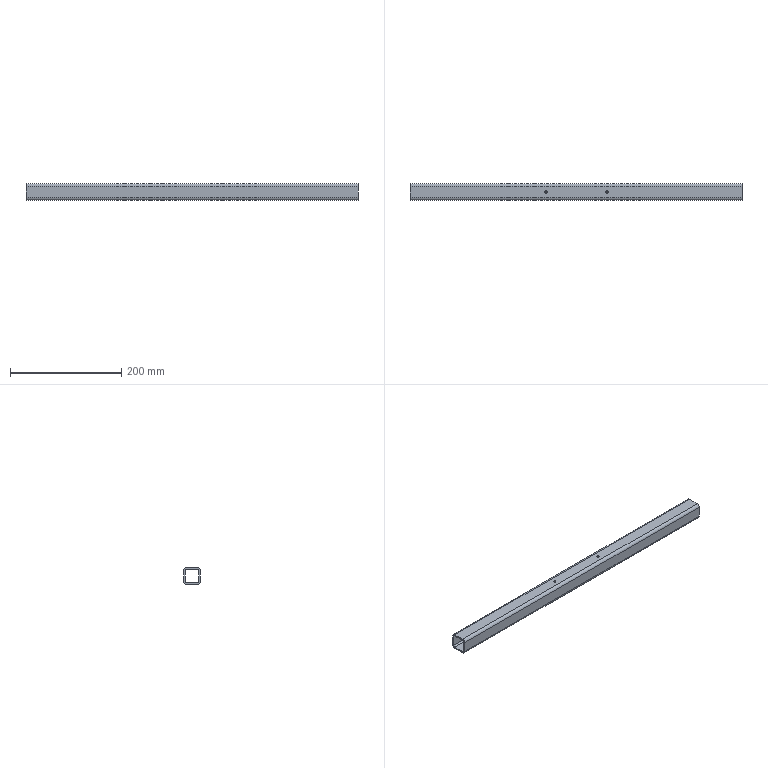Part | SolidWorks | features 3DProfileFeature 1, HoleWzd 1, WeldMemberFeat 1, WeldmentFeature 1 | 1 solid | 26 faces | box 598 x 30 x 30 mm | volume 159852 mm3 | cylinder 16 | plane 10 | commonest cylinder face diameters 4.2 x8 5.2 x4 10.4 x4
STEP:
#1=CARTESIAN_POINT('',(357.1,0.,12.4));
#2=VERTEX_POINT('',#1);
#3=CARTESIAN_POINT('',(352.9,0.,12.4));
#4=VERTEX_POINT('',#3);
#5=CARTESIAN_POINT('',(355.,0.,12.4));
#6=DIRECTION('',(0.,0.,-1.));
#7=DIRECTION('',(-1.,0.,0.));
#8=AXIS2_PLACEMENT_3D('',#5,#6,#7);
#9=CIRCLE('',#8,2.1);
#10=EDGE_CURVE('',#2,#4,#9,.T.);
#11=ORIENTED_EDGE('',*,*,#10,.T.);
#12=CARTESIAN_POINT('',(352.9,0.,15.));
#13=VERTEX_POINT('',#12);
#14=CARTESIAN_POINT('',(352.9,0.,15.));
#15=DIRECTION('',(0.,0.,1.));
#16=VECTOR('',#15,1000.);
#17=LINE('',#14,#16);
#18=EDGE_CURVE('',#4,#13,#17,.T.);
#19=ORIENTED_EDGE('',*,*,#18,.T.);
#20=CARTESIAN_POINT('',(357.1,0.,15.));
#21=VERTEX_POINT('',#20);
#22=CARTESIAN_POINT('',(355.,0.,15.));
#23=DIRECTION('',(0.,0.,1.));
#24=DIRECTION('',(1.,0.,0.));
#25=AXIS2_PLACEMENT_3D('',#22,#23,#24);
#26=CIRCLE('',#25,2.1);
#27=EDGE_CURVE('',#13,#21,#26,.T.);
#28=ORIENTED_EDGE('',*,*,#27,.T.);
#29=CARTESIAN_POINT('',(357.1,0.,15.));
#30=DIRECTION('',(0.,0.,1.));
#31=VECTOR('',#30,1000.);
#32=LINE('',#29,#31);
#33=EDGE_CURVE('',#2,#21,#32,.T.);
#34=ORIENTED_EDGE('',*,*,#33,.F.);
#35=EDGE_LOOP('',(#11,#19,#28,#34));
#36=FACE_OUTER_BOUND('',#35,.T.);
#37=CARTESIAN_POINT('',(355.,0.,15.));
#38=DIRECTION('',(0.,0.,1.));
#39=DIRECTION('',(1.,0.,0.));
#40=AXIS2_PLACEMENT_3D('',#37,#38,#39);
#41=CYLINDRICAL_SURFACE('',#40,2.1);
#42=ADVANCED_FACE('',(#36),#41,.F.);
#43=CARTESIAN_POINT('',(352.9,0.,-15.));
#44=VERTEX_POINT('',#43);
#45=CARTESIAN_POINT('',(357.1,0.,-15.));
#46=VERTEX_POINT('',#45);
#47=CARTESIAN_POINT('',(355.,0.,-15.));
#48=DIRECTION('',(0.,0.,1.));
#49=DIRECTION('',(1.,0.,0.));
#50=AXIS2_PLACEMENT_3D('',#47,#48,#49);
#51=CIRCLE('',#50,2.1);
#52=EDGE_CURVE('',#44,#46,#51,.T.);
#53=ORIENTED_EDGE('',*,*,#52,.F.);
#54=CARTESIAN_POINT('',(352.9,0.,-12.4));
#55=VERTEX_POINT('',#54);
#56=CARTESIAN_POINT('',(352.9,0.,15.));
#57=DIRECTION('',(0.,0.,1.));
#58=VECTOR('',#57,1000.);
#59=LINE('',#56,#58);
#60=EDGE_CURVE('',#44,#55,#59,.T.);
#61=ORIENTED_EDGE('',*,*,#60,.T.);
#62=CARTESIAN_POINT('',(357.1,0.,-12.4));
#63=VERTEX_POINT('',#62);
#64=CARTESIAN_POINT('',(355.,0.,-12.4));
#65=DIRECTION('',(0.,0.,1.));
#66=DIRECTION('',(1.,0.,0.));
#67=AXIS2_PLACEMENT_3D('',#64,#65,#66);
#68=CIRCLE('',#67,2.1);
#69=EDGE_CURVE('',#55,#63,#68,.T.);
#70=ORIENTED_EDGE('',*,*,#69,.T.);
#71=CARTESIAN_POINT('',(357.1,0.,15.));
#72=DIRECTION('',(0.,0.,1.));
#73=VECTOR('',#72,1000.);
#74=LINE('',#71,#73);
#75=EDGE_CURVE('',#46,#63,#74,.T.);
#76=ORIENTED_EDGE('',*,*,#75,.F.);
#77=EDGE_LOOP('',(#53,#61,#70,#76));
#78=FACE_OUTER_BOUND('',#77,.T.);
#79=CARTESIAN_POINT('',(355.,0.,15.));
#80=DIRECTION('',(0.,0.,1.));
#81=DIRECTION('',(1.,0.,0.));
#82=AXIS2_PLACEMENT_3D('',#79,#80,#81);
#83=CYLINDRICAL_SURFACE('',#82,2.1);
#84=ADVANCED_FACE('',(#78),#83,.F.);
#85=CARTESIAN_POINT('',(247.1,0.,12.4));
#86=VERTEX_POINT('',#85);
#87=CARTESIAN_POINT('',(242.9,0.,12.4));
#88=VERTEX_POINT('',#87);
#89=CARTESIAN_POINT('',(245.,0.,12.4));
#90=DIRECTION('',(0.,0.,-1.));
#91=DIRECTION('',(-1.,0.,0.));
#92=AXIS2_PLACEMENT_3D('',#89,#90,#91);
#93=CIRCLE('',#92,2.1);
#94=EDGE_CURVE('',#86,#88,#93,.T.);
#95=ORIENTED_EDGE('',*,*,#94,.T.);
#96=CARTESIAN_POINT('',(242.9,0.,15.));
#97=VERTEX_POINT('',#96);
#98=CARTESIAN_POINT('',(242.9,0.,15.));
#99=DIRECTION('',(0.,0.,1.));
#100=VECTOR('',#99,1000.);
#101=LINE('',#98,#100);
#102=EDGE_CURVE('',#88,#97,#101,.T.);
#103=ORIENTED_EDGE('',*,*,#102,.T.);
#104=CARTESIAN_POINT('',(247.1,0.,15.));
#105=VERTEX_POINT('',#104);
#106=CARTESIAN_POINT('',(245.,0.,15.));
#107=DIRECTION('',(0.,0.,1.));
#108=DIRECTION('',(1.,0.,0.));
#109=AXIS2_PLACEMENT_3D('',#106,#107,#108);
#110=CIRCLE('',#109,2.1);
#111=EDGE_CURVE('',#97,#105,#110,.T.);
#112=ORIENTED_EDGE('',*,*,#111,.T.);
#113=CARTESIAN_POINT('',(247.1,0.,15.));
#114=DIRECTION('',(0.,0.,1.));
#115=VECTOR('',#114,1000.);
#116=LINE('',#113,#115);
#117=EDGE_CURVE('',#86,#105,#116,.T.);
#118=ORIENTED_EDGE('',*,*,#117,.F.);
#119=EDGE_LOOP('',(#95,#103,#112,#118));
#120=FACE_OUTER_BOUND('',#119,.T.);
#121=CARTESIAN_POINT('',(245.,0.,15.));
#122=DIRECTION('',(0.,0.,1.));
#123=DIRECTION('',(1.,0.,0.));
#124=AXIS2_PLACEMENT_3D('',#121,#122,#123);
#125=CYLINDRICAL_SURFACE('',#124,2.1);
#126=ADVANCED_FACE('',(#120),#125,.F.);
#127=CARTESIAN_POINT('',(242.9,0.,-15.));
#128=VERTEX_POINT('',#127);
#129=CARTESIAN_POINT('',(247.1,0.,-15.));
#130=VERTEX_POINT('',#129);
#131=CARTESIAN_POINT('',(245.,0.,-15.));
#132=DIRECTION('',(0.,0.,1.));
#133=DIRECTION('',(1.,0.,0.));
#134=AXIS2_PLACEMENT_3D('',#131,#132,#133);
#135=CIRCLE('',#134,2.1);
#136=EDGE_CURVE('',#128,#130,#135,.T.);
#137=ORIENTED_EDGE('',*,*,#136,.F.);
#138=CARTESIAN_POINT('',(242.9,0.,-12.4));
#139=VERTEX_POINT('',#138);
#140=CARTESIAN_POINT('',(242.9,0.,15.));
#141=DIRECTION('',(0.,0.,1.));
#142=VECTOR('',#141,1000.);
#143=LINE('',#140,#142);
#144=EDGE_CURVE('',#128,#139,#143,.T.);
#145=ORIENTED_EDGE('',*,*,#144,.T.);
#146=CARTESIAN_POINT('',(247.1,0.,-12.4));
#147=VERTEX_POINT('',#146);
#148=CARTESIAN_POINT('',(245.,0.,-12.4));
#149=DIRECTION('',(0.,0.,1.));
#150=DIRECTION('',(1.,0.,0.));
#151=AXIS2_PLACEMENT_3D('',#148,#149,#150);
#152=CIRCLE('',#151,2.1);
#153=EDGE_CURVE('',#139,#147,#152,.T.);
#154=ORIENTED_EDGE('',*,*,#153,.T.);
#155=CARTESIAN_POINT('',(247.1,0.,15.));
#156=DIRECTION('',(0.,0.,1.));
#157=VECTOR('',#156,1000.);
#158=LINE('',#155,#157);
#159=EDGE_CURVE('',#130,#147,#158,.T.);
#160=ORIENTED_EDGE('',*,*,#159,.F.);
#161=EDGE_LOOP('',(#137,#145,#154,#160));
#162=FACE_OUTER_BOUND('',#161,.T.);
#163=CARTESIAN_POINT('',(245.,0.,15.));
#164=DIRECTION('',(0.,0.,1.));
#165=DIRECTION('',(1.,0.,0.));
#166=AXIS2_PLACEMENT_3D('',#163,#164,#165);
#167=CYLINDRICAL_SURFACE('',#166,2.1);
#168=ADVANCED_FACE('',(#162),#167,.F.);
#169=CARTESIAN_POINT('',(0.,9.8,-15.));
#170=VERTEX_POINT('',#169);
#171=CARTESIAN_POINT('',(0.,15.,-9.8));
#172=VERTEX_POINT('',#171);
#173=CARTESIAN_POINT('',(0.,9.8,-9.8));
#174=DIRECTION('',(1.,0.,0.));
#175=DIRECTION('',(0.,0.,-1.));
#176=AXIS2_PLACEMENT_3D('',#173,#174,#175);
#177=CIRCLE('',#176,5.2);
#178=EDGE_CURVE('',#170,#172,#177,.T.);
#179=ORIENTED_EDGE('',*,*,#178,.T.);
#180=CARTESIAN_POINT('',(598.,15.,-9.8));
#181=VERTEX_POINT('',#180);
#182=CARTESIAN_POINT('',(598.,15.,-9.8));
#183=DIRECTION('',(-1.,0.,0.));
#184=VECTOR('',#183,1000.);
#185=LINE('',#182,#184);
#186=EDGE_CURVE('',#181,#172,#185,.T.);
#187=ORIENTED_EDGE('',*,*,#186,.F.);
#188=CARTESIAN_POINT('',(598.,9.8,-15.));
#189=VERTEX_POINT('',#188);
#190=CARTESIAN_POINT('',(598.,9.8,-9.8));
#191=DIRECTION('',(1.,0.,0.));
#192=DIRECTION('',(0.,0.,-1.));
#193=AXIS2_PLACEMENT_3D('',#190,#191,#192);
#194=CIRCLE('',#193,5.2);
#195=EDGE_CURVE('',#189,#181,#194,.T.);
#196=ORIENTED_EDGE('',*,*,#195,.F.);
#197=CARTESIAN_POINT('',(598.,9.8,-15.));
#198=DIRECTION('',(-1.,0.,0.));
#199=VECTOR('',#198,1000.);
#200=LINE('',#197,#199);
#201=EDGE_CURVE('',#189,#170,#200,.T.);
#202=ORIENTED_EDGE('',*,*,#201,.T.);
#203=EDGE_LOOP('',(#179,#187,#196,#202));
#204=FACE_OUTER_BOUND('',#203,.T.);
#205=CARTESIAN_POINT('',(598.,9.8,-9.8));
#206=DIRECTION('',(-1.,0.,0.));
#207=DIRECTION('',(0.,0.,1.));
#208=AXIS2_PLACEMENT_3D('',#205,#206,#207);
#209=CYLINDRICAL_SURFACE('',#208,5.2);
#210=ADVANCED_FACE('',(#204),#209,.T.);
#211=CARTESIAN_POINT('',(0.,15.,9.8));
#212=VERTEX_POINT('',#211);
#213=CARTESIAN_POINT('',(0.,15.,-9.8));
#214=DIRECTION('',(0.,0.,1.));
#215=VECTOR('',#214,1000.);
#216=LINE('',#213,#215);
#217=EDGE_CURVE('',#172,#212,#216,.T.);
#218=ORIENTED_EDGE('',*,*,#217,.T.);
#219=CARTESIAN_POINT('',(598.,15.,9.8));
#220=VERTEX_POINT('',#219);
#221=CARTESIAN_POINT('',(598.,15.,9.8));
#222=DIRECTION('',(-1.,0.,0.));
#223=VECTOR('',#222,1000.);
#224=LINE('',#221,#223);
#225=EDGE_CURVE('',#220,#212,#224,.T.);
#226=ORIENTED_EDGE('',*,*,#225,.F.);
#227=CARTESIAN_POINT('',(598.,15.,-9.8));
#228=DIRECTION('',(0.,0.,1.));
#229=VECTOR('',#228,1000.);
#230=LINE('',#227,#229);
#231=EDGE_CURVE('',#181,#220,#230,.T.);
#232=ORIENTED_EDGE('',*,*,#231,.F.);
#233=ORIENTED_EDGE('',*,*,#186,.T.);
#234=EDGE_LOOP('',(#218,#226,#232,#233));
#235=FACE_OUTER_BOUND('',#234,.T.);
#236=CARTESIAN_POINT('',(598.,15.,-9.8));
#237=DIRECTION('',(0.,-1.,0.));
#238=DIRECTION('',(0.,0.,-1.));
#239=AXIS2_PLACEMENT_3D('',#236,#237,#238);
#240=PLANE('',#239);
#241=ADVANCED_FACE('',(#235),#240,.F.);
#242=CARTESIAN_POINT('',(0.,9.8,15.));
#243=VERTEX_POINT('',#242);
#244=CARTESIAN_POINT('',(0.,9.8,9.8));
#245=DIRECTION('',(1.,0.,0.));
#246=DIRECTION('',(0.,0.,-1.));
#247=AXIS2_PLACEMENT_3D('',#244,#245,#246);
#248=CIRCLE('',#247,5.2);
#249=EDGE_CURVE('',#212,#243,#248,.T.);
#250=ORIENTED_EDGE('',*,*,#249,.T.);
#251=CARTESIAN_POINT('',(598.,9.8,15.));
#252=VERTEX_POINT('',#251);
#253=CARTESIAN_POINT('',(598.,9.8,15.));
#254=DIRECTION('',(-1.,0.,0.));
#255=VECTOR('',#254,1000.);
#256=LINE('',#253,#255);
#257=EDGE_CURVE('',#252,#243,#256,.T.);
#258=ORIENTED_EDGE('',*,*,#257,.F.);
#259=CARTESIAN_POINT('',(598.,9.8,9.8));
#260=DIRECTION('',(1.,0.,0.));
#261=DIRECTION('',(0.,0.,-1.));
#262=AXIS2_PLACEMENT_3D('',#259,#260,#261);
#263=CIRCLE('',#262,5.2);
#264=EDGE_CURVE('',#220,#252,#263,.T.);
#265=ORIENTED_EDGE('',*,*,#264,.F.);
#266=ORIENTED_EDGE('',*,*,#225,.T.);
#267=EDGE_LOOP('',(#250,#258,#265,#266));
#268=FACE_OUTER_BOUND('',#267,.T.);
#269=CARTESIAN_POINT('',(598.,9.8,9.8));
#270=DIRECTION('',(-1.,0.,0.));
#271=DIRECTION('',(0.,0.,1.));
#272=AXIS2_PLACEMENT_3D('',#269,#270,#271);
#273=CYLINDRICAL_SURFACE('',#272,5.2);
#274=ADVANCED_FACE('',(#268),#273,.T.);
#275=CARTESIAN_POINT('',(355.,0.,15.));
#276=DIRECTION('',(0.,0.,1.));
#277=DIRECTION('',(1.,0.,0.));
#278=AXIS2_PLACEMENT_3D('',#275,#276,#277);
#279=CIRCLE('',#278,2.1);
#280=EDGE_CURVE('',#21,#13,#279,.T.);
#281=ORIENTED_EDGE('',*,*,#280,.F.);
#282=ORIENTED_EDGE('',*,*,#27,.F.);
#283=EDGE_LOOP('',(#281,#282));
#284=FACE_BOUND('',#283,.T.);
#285=CARTESIAN_POINT('',(245.,0.,15.));
#286=DIRECTION('',(0.,0.,1.));
#287=DIRECTION('',(1.,0.,0.));
#288=AXIS2_PLACEMENT_3D('',#285,#286,#287);
#289=CIRCLE('',#288,2.1);
#290=EDGE_CURVE('',#105,#97,#289,.T.);
#291=ORIENTED_EDGE('',*,*,#290,.F.);
#292=ORIENTED_EDGE('',*,*,#111,.F.);
#293=EDGE_LOOP('',(#291,#292));
#294=FACE_BOUND('',#293,.T.);
#295=CARTESIAN_POINT('',(0.,-9.8,15.));
#296=VERTEX_POINT('',#295);
#297=CARTESIAN_POINT('',(0.,-9.8,15.));
#298=DIRECTION('',(0.,-1.,0.));
#299=VECTOR('',#298,1000.);
#300=LINE('',#297,#299);
#301=EDGE_CURVE('',#243,#296,#300,.T.);
#302=ORIENTED_EDGE('',*,*,#301,.T.);
#303=CARTESIAN_POINT('',(598.,-9.8,15.));
#304=VERTEX_POINT('',#303);
#305=CARTESIAN_POINT('',(598.,-9.8,15.));
#306=DIRECTION('',(-1.,0.,0.));
#307=VECTOR('',#306,1000.);
#308=LINE('',#305,#307);
#309=EDGE_CURVE('',#304,#296,#308,.T.);
#310=ORIENTED_EDGE('',*,*,#309,.F.);
#311=CARTESIAN_POINT('',(598.,-9.8,15.));
#312=DIRECTION('',(0.,-1.,0.));
#313=VECTOR('',#312,1000.);
#314=LINE('',#311,#313);
#315=EDGE_CURVE('',#252,#304,#314,.T.);
#316=ORIENTED_EDGE('',*,*,#315,.F.);
#317=ORIENTED_EDGE('',*,*,#257,.T.);
#318=EDGE_LOOP('',(#302,#310,#316,#317));
#319=FACE_OUTER_BOUND('',#318,.T.);
#320=CARTESIAN_POINT('',(598.,-9.8,15.));
#321=DIRECTION('',(0.,0.,-1.));
#322=DIRECTION('',(-1.,0.,0.));
#323=AXIS2_PLACEMENT_3D('',#320,#321,#322);
#324=PLANE('',#323);
#325=ADVANCED_FACE('',(#284,#294,#319),#324,.F.);
#326=CARTESIAN_POINT('',(0.,-15.,9.8));
#327=VERTEX_POINT('',#326);
#328=CARTESIAN_POINT('',(0.,-9.8,9.8));
#329=DIRECTION('',(1.,0.,0.));
#330=DIRECTION('',(0.,0.,-1.));
#331=AXIS2_PLACEMENT_3D('',#328,#329,#330);
#332=CIRCLE('',#331,5.2);
#333=EDGE_CURVE('',#296,#327,#332,.T.);
#334=ORIENTED_EDGE('',*,*,#333,.T.);
#335=CARTESIAN_POINT('',(598.,-15.,9.8));
#336=VERTEX_POINT('',#335);
#337=CARTESIAN_POINT('',(598.,-15.,9.8));
#338=DIRECTION('',(-1.,0.,0.));
#339=VECTOR('',#338,1000.);
#340=LINE('',#337,#339);
#341=EDGE_CURVE('',#336,#327,#340,.T.);
#342=ORIENTED_EDGE('',*,*,#341,.F.);
#343=CARTESIAN_POINT('',(598.,-9.8,9.8));
#344=DIRECTION('',(1.,0.,0.));
#345=DIRECTION('',(0.,0.,-1.));
#346=AXIS2_PLACEMENT_3D('',#343,#344,#345);
#347=CIRCLE('',#346,5.2);
#348=EDGE_CURVE('',#304,#336,#347,.T.);
#349=ORIENTED_EDGE('',*,*,#348,.F.);
#350=ORIENTED_EDGE('',*,*,#309,.T.);
#351=EDGE_LOOP('',(#334,#342,#349,#350));
#352=FACE_OUTER_BOUND('',#351,.T.);
#353=CARTESIAN_POINT('',(598.,-9.8,9.8));
#354=DIRECTION('',(-1.,0.,0.));
#355=DIRECTION('',(0.,0.,1.));
#356=AXIS2_PLACEMENT_3D('',#353,#354,#355);
#357=CYLINDRICAL_SURFACE('',#356,5.2);
#358=ADVANCED_FACE('',(#352),#357,.T.);
#359=CARTESIAN_POINT('',(0.,-15.,-9.8));
#360=VERTEX_POINT('',#359);
#361=CARTESIAN_POINT('',(0.,-15.,9.8));
#362=DIRECTION('',(0.,0.,-1.));
#363=VECTOR('',#362,1000.);
#364=LINE('',#361,#363);
#365=EDGE_CURVE('',#327,#360,#364,.T.);
#366=ORIENTED_EDGE('',*,*,#365,.T.);
#367=CARTESIAN_POINT('',(598.,-15.,-9.8));
#368=VERTEX_POINT('',#367);
#369=CARTESIAN_POINT('',(598.,-15.,-9.8));
#370=DIRECTION('',(-1.,0.,0.));
#371=VECTOR('',#370,1000.);
#372=LINE('',#369,#371);
#373=EDGE_CURVE('',#368,#360,#372,.T.);
#374=ORIENTED_EDGE('',*,*,#373,.F.);
#375=CARTESIAN_POINT('',(598.,-15.,9.8));
#376=DIRECTION('',(0.,0.,-1.));
#377=VECTOR('',#376,1000.);
#378=LINE('',#375,#377);
#379=EDGE_CURVE('',#336,#368,#378,.T.);
#380=ORIENTED_EDGE('',*,*,#379,.F.);
#381=ORIENTED_EDGE('',*,*,#341,.T.);
#382=EDGE_LOOP('',(#366,#374,#380,#381));
#383=FACE_OUTER_BOUND('',#382,.T.);
#384=CARTESIAN_POINT('',(598.,-15.,9.8));
#385=DIRECTION('',(0.,1.,0.));
#386=DIRECTION('',(0.,0.,1.));
#387=AXIS2_PLACEMENT_3D('',#384,#385,#386);
#388=PLANE('',#387);
#389=ADVANCED_FACE('',(#383),#388,.F.);
#390=CARTESIAN_POINT('',(0.,-9.8,-15.));
#391=VERTEX_POINT('',#390);
#392=CARTESIAN_POINT('',(0.,-9.8,-9.8));
#393=DIRECTION('',(1.,0.,0.));
#394=DIRECTION('',(0.,0.,-1.));
#395=AXIS2_PLACEMENT_3D('',#392,#393,#394);
#396=CIRCLE('',#395,5.2);
#397=EDGE_CURVE('',#360,#391,#396,.T.);
#398=ORIENTED_EDGE('',*,*,#397,.T.);
#399=CARTESIAN_POINT('',(598.,-9.8,-15.));
#400=VERTEX_POINT('',#399);
#401=CARTESIAN_POINT('',(598.,-9.8,-15.));
#402=DIRECTION('',(-1.,0.,0.));
#403=VECTOR('',#402,1000.);
#404=LINE('',#401,#403);
#405=EDGE_CURVE('',#400,#391,#404,.T.);
#406=ORIENTED_EDGE('',*,*,#405,.F.);
#407=CARTESIAN_POINT('',(598.,-9.8,-9.8));
#408=DIRECTION('',(1.,0.,0.));
#409=DIRECTION('',(0.,0.,-1.));
#410=AXIS2_PLACEMENT_3D('',#407,#408,#409);
#411=CIRCLE('',#410,5.2);
#412=EDGE_CURVE('',#368,#400,#411,.T.);
#413=ORIENTED_EDGE('',*,*,#412,.F.);
#414=ORIENTED_EDGE('',*,*,#373,.T.);
#415=EDGE_LOOP('',(#398,#406,#413,#414));
#416=FACE_OUTER_BOUND('',#415,.T.);
#417=CARTESIAN_POINT('',(598.,-9.8,-9.8));
#418=DIRECTION('',(-1.,0.,0.));
#419=DIRECTION('',(0.,0.,1.));
#420=AXIS2_PLACEMENT_3D('',#417,#418,#419);
#421=CYLINDRICAL_SURFACE('',#420,5.2);
#422=ADVANCED_FACE('',(#416),#421,.T.);
#423=CARTESIAN_POINT('',(0.,12.4,9.8));
#424=VERTEX_POINT('',#423);
#425=CARTESIAN_POINT('',(0.,9.8,12.4));
#426=VERTEX_POINT('',#425);
#427=CARTESIAN_POINT('',(0.,9.8,9.8));
#428=DIRECTION('',(1.,0.,0.));
#429=DIRECTION('',(0.,0.,-1.));
#430=AXIS2_PLACEMENT_3D('',#427,#428,#429);
#431=CIRCLE('',#430,2.6);
#432=EDGE_CURVE('',#424,#426,#431,.T.);
#433=ORIENTED_EDGE('',*,*,#432,.F.);
#434=CARTESIAN_POINT('',(598.,12.4,9.8));
#435=VERTEX_POINT('',#434);
#436=CARTESIAN_POINT('',(598.,12.4,9.8));
#437=DIRECTION('',(-1.,0.,0.));
#438=VECTOR('',#437,1000.);
#439=LINE('',#436,#438);
#440=EDGE_CURVE('',#435,#424,#439,.T.);
#441=ORIENTED_EDGE('',*,*,#440,.F.);
#442=CARTESIAN_POINT('',(598.,9.8,12.4));
#443=VERTEX_POINT('',#442);
#444=CARTESIAN_POINT('',(598.,9.8,9.8));
#445=DIRECTION('',(1.,0.,0.));
#446=DIRECTION('',(0.,0.,-1.));
#447=AXIS2_PLACEMENT_3D('',#444,#445,#446);
#448=CIRCLE('',#447,2.6);
#449=EDGE_CURVE('',#435,#443,#448,.T.);
#450=ORIENTED_EDGE('',*,*,#449,.T.);
#451=CARTESIAN_POINT('',(598.,9.8,12.4));
#452=DIRECTION('',(-1.,0.,0.));
#453=VECTOR('',#452,1000.);
#454=LINE('',#451,#453);
#455=EDGE_CURVE('',#443,#426,#454,.T.);
#456=ORIENTED_EDGE('',*,*,#455,.T.);
#457=EDGE_LOOP('',(#433,#441,#450,#456));
#458=FACE_OUTER_BOUND('',#457,.T.);
#459=CARTESIAN_POINT('',(598.,9.8,9.8));
#460=DIRECTION('',(-1.,0.,0.));
#461=DIRECTION('',(0.,0.,1.));
#462=AXIS2_PLACEMENT_3D('',#459,#460,#461);
#463=CYLINDRICAL_SURFACE('',#462,2.6);
#464=ADVANCED_FACE('',(#458),#463,.F.);
#465=CARTESIAN_POINT('',(0.,12.4,-9.8));
#466=VERTEX_POINT('',#465);
#467=CARTESIAN_POINT('',(0.,12.4,-9.8));
#468=DIRECTION('',(0.,0.,1.));
#469=VECTOR('',#468,1000.);
#470=LINE('',#467,#469);
#471=EDGE_CURVE('',#466,#424,#470,.T.);
#472=ORIENTED_EDGE('',*,*,#471,.F.);
#473=CARTESIAN_POINT('',(598.,12.4,-9.8));
#474=VERTEX_POINT('',#473);
#475=CARTESIAN_POINT('',(598.,12.4,-9.8));
#476=DIRECTION('',(-1.,0.,0.));
#477=VECTOR('',#476,1000.);
#478=LINE('',#475,#477);
#479=EDGE_CURVE('',#474,#466,#478,.T.);
#480=ORIENTED_EDGE('',*,*,#479,.F.);
#481=CARTESIAN_POINT('',(598.,12.4,-9.8));
#482=DIRECTION('',(0.,0.,1.));
#483=VECTOR('',#482,1000.);
#484=LINE('',#481,#483);
#485=EDGE_CURVE('',#474,#435,#484,.T.);
#486=ORIENTED_EDGE('',*,*,#485,.T.);
#487=ORIENTED_EDGE('',*,*,#440,.T.);
#488=EDGE_LOOP('',(#472,#480,#486,#487));
#489=FACE_OUTER_BOUND('',#488,.T.);
#490=CARTESIAN_POINT('',(598.,12.4,-9.8));
#491=DIRECTION('',(0.,-1.,0.));
#492=DIRECTION('',(0.,0.,-1.));
#493=AXIS2_PLACEMENT_3D('',#490,#491,#492);
#494=PLANE('',#493);
#495=ADVANCED_FACE('',(#489),#494,.T.);
#496=CARTESIAN_POINT('',(0.,9.8,-12.4));
#497=VERTEX_POINT('',#496);
#498=CARTESIAN_POINT('',(0.,9.8,-9.8));
#499=DIRECTION('',(1.,0.,0.));
#500=DIRECTION('',(0.,0.,-1.));
#501=AXIS2_PLACEMENT_3D('',#498,#499,#500);
#502=CIRCLE('',#501,2.6);
#503=EDGE_CURVE('',#497,#466,#502,.T.);
#504=ORIENTED_EDGE('',*,*,#503,.F.);
#505=CARTESIAN_POINT('',(598.,9.8,-12.4));
#506=VERTEX_POINT('',#505);
#507=CARTESIAN_POINT('',(598.,9.8,-12.4));
#508=DIRECTION('',(-1.,0.,0.));
#509=VECTOR('',#508,1000.);
#510=LINE('',#507,#509);
#511=EDGE_CURVE('',#506,#497,#510,.T.);
#512=ORIENTED_EDGE('',*,*,#511,.F.);
#513=CARTESIAN_POINT('',(598.,9.8,-9.8));
#514=DIRECTION('',(1.,0.,0.));
#515=DIRECTION('',(0.,0.,-1.));
#516=AXIS2_PLACEMENT_3D('',#513,#514,#515);
#517=CIRCLE('',#516,2.6);
#518=EDGE_CURVE('',#506,#474,#517,.T.);
#519=ORIENTED_EDGE('',*,*,#518,.T.);
#520=ORIENTED_EDGE('',*,*,#479,.T.);
#521=EDGE_LOOP('',(#504,#512,#519,#520));
#522=FACE_OUTER_BOUND('',#521,.T.);
#523=CARTESIAN_POINT('',(598.,9.8,-9.8));
#524=DIRECTION('',(-1.,0.,0.));
#525=DIRECTION('',(0.,0.,1.));
#526=AXIS2_PLACEMENT_3D('',#523,#524,#525);
#527=CYLINDRICAL_SURFACE('',#526,2.6);
#528=ADVANCED_FACE('',(#522),#527,.F.);
#529=CARTESIAN_POINT('',(355.,0.,-12.4));
#530=DIRECTION('',(0.,0.,1.));
#531=DIRECTION('',(1.,0.,0.));
#532=AXIS2_PLACEMENT_3D('',#529,#530,#531);
#533=CIRCLE('',#532,2.1);
#534=EDGE_CURVE('',#63,#55,#533,.T.);
#535=ORIENTED_EDGE('',*,*,#534,.F.);
#536=ORIENTED_EDGE('',*,*,#69,.F.);
#537=EDGE_LOOP('',(#535,#536));
#538=FACE_BOUND('',#537,.T.);
#539=CARTESIAN_POINT('',(245.,0.,-12.4));
#540=DIRECTION('',(0.,0.,1.));
#541=DIRECTION('',(1.,0.,0.));
#542=AXIS2_PLACEMENT_3D('',#539,#540,#541);
#543=CIRCLE('',#542,2.1);
#544=EDGE_CURVE('',#147,#139,#543,.T.);
#545=ORIENTED_EDGE('',*,*,#544,.F.);
#546=ORIENTED_EDGE('',*,*,#153,.F.);
#547=EDGE_LOOP('',(#545,#546));
#548=FACE_BOUND('',#547,.T.);
#549=CARTESIAN_POINT('',(0.,-9.8,-12.4));
#550=VERTEX_POINT('',#549);
#551=CARTESIAN_POINT('',(0.,9.8,-12.4));
#552=DIRECTION('',(0.,1.,0.));
#553=VECTOR('',#552,1000.);
#554=LINE('',#551,#553);
#555=EDGE_CURVE('',#550,#497,#554,.T.);
#556=ORIENTED_EDGE('',*,*,#555,.F.);
#557=CARTESIAN_POINT('',(598.,-9.8,-12.4));
#558=VERTEX_POINT('',#557);
#559=CARTESIAN_POINT('',(598.,-9.8,-12.4));
#560=DIRECTION('',(-1.,0.,0.));
#561=VECTOR('',#560,1000.);
#562=LINE('',#559,#561);
#563=EDGE_CURVE('',#558,#550,#562,.T.);
#564=ORIENTED_EDGE('',*,*,#563,.F.);
#565=CARTESIAN_POINT('',(598.,9.8,-12.4));
#566=DIRECTION('',(0.,1.,0.));
#567=VECTOR('',#566,1000.);
#568=LINE('',#565,#567);
#569=EDGE_CURVE('',#558,#506,#568,.T.);
#570=ORIENTED_EDGE('',*,*,#569,.T.);
#571=ORIENTED_EDGE('',*,*,#511,.T.);
#572=EDGE_LOOP('',(#556,#564,#570,#571));
#573=FACE_OUTER_BOUND('',#572,.T.);
#574=CARTESIAN_POINT('',(598.,9.8,-12.4));
#575=DIRECTION('',(0.,0.,1.));
#576=DIRECTION('',(1.,0.,0.));
#577=AXIS2_PLACEMENT_3D('',#574,#575,#576);
#578=PLANE('',#577);
#579=ADVANCED_FACE('',(#538,#548,#573),#578,.T.);
#580=CARTESIAN_POINT('',(0.,-12.4,-9.8));
#581=VERTEX_POINT('',#580);
#582=CARTESIAN_POINT('',(0.,-9.8,-9.8));
#583=DIRECTION('',(1.,0.,0.));
#584=DIRECTION('',(0.,0.,-1.));
#585=AXIS2_PLACEMENT_3D('',#582,#583,#584);
#586=CIRCLE('',#585,2.6);
#587=EDGE_CURVE('',#581,#550,#586,.T.);
#588=ORIENTED_EDGE('',*,*,#587,.F.);
#589=CARTESIAN_POINT('',(598.,-12.4,-9.8));
#590=VERTEX_POINT('',#589);
#591=CARTESIAN_POINT('',(598.,-12.4,-9.8));
#592=DIRECTION('',(-1.,0.,0.));
#593=VECTOR('',#592,1000.);
#594=LINE('',#591,#593);
#595=EDGE_CURVE('',#590,#581,#594,.T.);
#596=ORIENTED_EDGE('',*,*,#595,.F.);
#597=CARTESIAN_POINT('',(598.,-9.8,-9.8));
#598=DIRECTION('',(1.,0.,0.));
#599=DIRECTION('',(0.,0.,-1.));
#600=AXIS2_PLACEMENT_3D('',#597,#598,#599);
#601=CIRCLE('',#600,2.6);
#602=EDGE_CURVE('',#590,#558,#601,.T.);
#603=ORIENTED_EDGE('',*,*,#602,.T.);
#604=ORIENTED_EDGE('',*,*,#563,.T.);
#605=EDGE_LOOP('',(#588,#596,#603,#604));
#606=FACE_OUTER_BOUND('',#605,.T.);
#607=CARTESIAN_POINT('',(598.,-9.8,-9.8));
#608=DIRECTION('',(-1.,0.,0.));
#609=DIRECTION('',(0.,0.,1.));
#610=AXIS2_PLACEMENT_3D('',#607,#608,#609);
#611=CYLINDRICAL_SURFACE('',#610,2.6);
#612=ADVANCED_FACE('',(#606),#611,.F.);
#613=CARTESIAN_POINT('',(0.,-12.4,9.8));
#614=VERTEX_POINT('',#613);
#615=CARTESIAN_POINT('',(0.,-12.4,9.8));
#616=DIRECTION('',(0.,0.,-1.));
#617=VECTOR('',#616,1000.);
#618=LINE('',#615,#617);
#619=EDGE_CURVE('',#614,#581,#618,.T.);
#620=ORIENTED_EDGE('',*,*,#619,.F.);
#621=CARTESIAN_POINT('',(598.,-12.4,9.8));
#622=VERTEX_POINT('',#621);
#623=CARTESIAN_POINT('',(598.,-12.4,9.8));
#624=DIRECTION('',(-1.,0.,0.));
#625=VECTOR('',#624,1000.);
#626=LINE('',#623,#625);
#627=EDGE_CURVE('',#622,#614,#626,.T.);
#628=ORIENTED_EDGE('',*,*,#627,.F.);
#629=CARTESIAN_POINT('',(598.,-12.4,9.8));
#630=DIRECTION('',(0.,0.,-1.));
#631=VECTOR('',#630,1000.);
#632=LINE('',#629,#631);
#633=EDGE_CURVE('',#622,#590,#632,.T.);
#634=ORIENTED_EDGE('',*,*,#633,.T.);
#635=ORIENTED_EDGE('',*,*,#595,.T.);
#636=EDGE_LOOP('',(#620,#628,#634,#635));
#637=FACE_OUTER_BOUND('',#636,.T.);
#638=CARTESIAN_POINT('',(598.,-12.4,9.8));
#639=DIRECTION('',(0.,1.,0.));
#640=DIRECTION('',(0.,0.,1.));
#641=AXIS2_PLACEMENT_3D('',#638,#639,#640);
#642=PLANE('',#641);
#643=ADVANCED_FACE('',(#637),#642,.T.);
#644=CARTESIAN_POINT('',(0.,-9.8,12.4));
#645=VERTEX_POINT('',#644);
#646=CARTESIAN_POINT('',(0.,-9.8,9.8));
#647=DIRECTION('',(1.,0.,0.));
#648=DIRECTION('',(0.,0.,-1.));
#649=AXIS2_PLACEMENT_3D('',#646,#647,#648);
#650=CIRCLE('',#649,2.6);
#651=EDGE_CURVE('',#645,#614,#650,.T.);
#652=ORIENTED_EDGE('',*,*,#651,.F.);
#653=CARTESIAN_POINT('',(598.,-9.8,12.4));
#654=VERTEX_POINT('',#653);
#655=CARTESIAN_POINT('',(598.,-9.8,12.4));
#656=DIRECTION('',(-1.,0.,0.));
#657=VECTOR('',#656,1000.);
#658=LINE('',#655,#657);
#659=EDGE_CURVE('',#654,#645,#658,.T.);
#660=ORIENTED_EDGE('',*,*,#659,.F.);
#661=CARTESIAN_POINT('',(598.,-9.8,9.8));
#662=DIRECTION('',(1.,0.,0.));
#663=DIRECTION('',(0.,0.,-1.));
#664=AXIS2_PLACEMENT_3D('',#661,#662,#663);
#665=CIRCLE('',#664,2.6);
#666=EDGE_CURVE('',#654,#622,#665,.T.);
#667=ORIENTED_EDGE('',*,*,#666,.T.);
#668=ORIENTED_EDGE('',*,*,#627,.T.);
#669=EDGE_LOOP('',(#652,#660,#667,#668));
#670=FACE_OUTER_BOUND('',#669,.T.);
#671=CARTESIAN_POINT('',(598.,-9.8,9.8));
#672=DIRECTION('',(-1.,0.,0.));
#673=DIRECTION('',(0.,0.,1.));
#674=AXIS2_PLACEMENT_3D('',#671,#672,#673);
#675=CYLINDRICAL_SURFACE('',#674,2.6);
#676=ADVANCED_FACE('',(#670),#675,.F.);
#677=ORIENTED_EDGE('',*,*,#10,.F.);
#678=CARTESIAN_POINT('',(355.,0.,12.4));
#679=DIRECTION('',(0.,0.,-1.));
#680=DIRECTION('',(-1.,0.,0.));
#681=AXIS2_PLACEMENT_3D('',#678,#679,#680);
#682=CIRCLE('',#681,2.1);
#683=EDGE_CURVE('',#4,#2,#682,.T.);
#684=ORIENTED_EDGE('',*,*,#683,.F.);
#685=EDGE_LOOP('',(#677,#684));
#686=FACE_BOUND('',#685,.T.);
#687=ORIENTED_EDGE('',*,*,#94,.F.);
#688=CARTESIAN_POINT('',(245.,0.,12.4));
#689=DIRECTION('',(0.,0.,-1.));
#690=DIRECTION('',(-1.,0.,0.));
#691=AXIS2_PLACEMENT_3D('',#688,#689,#690);
#692=CIRCLE('',#691,2.1);
#693=EDGE_CURVE('',#88,#86,#692,.T.);
#694=ORIENTED_EDGE('',*,*,#693,.F.);
#695=EDGE_LOOP('',(#687,#694));
#696=FACE_BOUND('',#695,.T.);
#697=CARTESIAN_POINT('',(0.,-9.8,12.4));
#698=DIRECTION('',(0.,-1.,0.));
#699=VECTOR('',#698,1000.);
#700=LINE('',#697,#699);
#701=EDGE_CURVE('',#426,#645,#700,.T.);
#702=ORIENTED_EDGE('',*,*,#701,.F.);
#703=ORIENTED_EDGE('',*,*,#455,.F.);
#704=CARTESIAN_POINT('',(598.,-9.8,12.4));
#705=DIRECTION('',(0.,-1.,0.));
#706=VECTOR('',#705,1000.);
#707=LINE('',#704,#706);
#708=EDGE_CURVE('',#443,#654,#707,.T.);
#709=ORIENTED_EDGE('',*,*,#708,.T.);
#710=ORIENTED_EDGE('',*,*,#659,.T.);
#711=EDGE_LOOP('',(#702,#703,#709,#710));
#712=FACE_OUTER_BOUND('',#711,.T.);
#713=CARTESIAN_POINT('',(598.,-9.8,12.4));
#714=DIRECTION('',(0.,0.,-1.));
#715=DIRECTION('',(-1.,0.,0.));
#716=AXIS2_PLACEMENT_3D('',#713,#714,#715);
#717=PLANE('',#716);
#718=ADVANCED_FACE('',(#686,#696,#712),#717,.T.);
#719=CARTESIAN_POINT('',(355.,0.,-15.));
#720=DIRECTION('',(0.,0.,1.));
#721=DIRECTION('',(1.,0.,0.));
#722=AXIS2_PLACEMENT_3D('',#719,#720,#721);
#723=CIRCLE('',#722,2.1);
#724=EDGE_CURVE('',#46,#44,#723,.T.);
#725=ORIENTED_EDGE('',*,*,#724,.T.);
#726=ORIENTED_EDGE('',*,*,#52,.T.);
#727=EDGE_LOOP('',(#725,#726));
#728=FACE_BOUND('',#727,.T.);
#729=CARTESIAN_POINT('',(245.,0.,-15.));
#730=DIRECTION('',(0.,0.,1.));
#731=DIRECTION('',(1.,0.,0.));
#732=AXIS2_PLACEMENT_3D('',#729,#730,#731);
#733=CIRCLE('',#732,2.1);
#734=EDGE_CURVE('',#130,#128,#733,.T.);
#735=ORIENTED_EDGE('',*,*,#734,.T.);
#736=ORIENTED_EDGE('',*,*,#136,.T.);
#737=EDGE_LOOP('',(#735,#736));
#738=FACE_BOUND('',#737,.T.);
#739=CARTESIAN_POINT('',(0.,9.8,-15.));
#740=DIRECTION('',(0.,1.,0.));
#741=VECTOR('',#740,1000.);
#742=LINE('',#739,#741);
#743=EDGE_CURVE('',#391,#170,#742,.T.);
#744=ORIENTED_EDGE('',*,*,#743,.T.);
#745=ORIENTED_EDGE('',*,*,#201,.F.);
#746=CARTESIAN_POINT('',(598.,9.8,-15.));
#747=DIRECTION('',(0.,1.,0.));
#748=VECTOR('',#747,1000.);
#749=LINE('',#746,#748);
#750=EDGE_CURVE('',#400,#189,#749,.T.);
#751=ORIENTED_EDGE('',*,*,#750,.F.);
#752=ORIENTED_EDGE('',*,*,#405,.T.);
#753=EDGE_LOOP('',(#744,#745,#751,#752));
#754=FACE_OUTER_BOUND('',#753,.T.);
#755=CARTESIAN_POINT('',(598.,9.8,-15.));
#756=DIRECTION('',(0.,0.,1.));
#757=DIRECTION('',(1.,0.,0.));
#758=AXIS2_PLACEMENT_3D('',#755,#756,#757);
#759=PLANE('',#758);
#760=ADVANCED_FACE('',(#728,#738,#754),#759,.F.);
#761=ORIENTED_EDGE('',*,*,#449,.F.);
#762=ORIENTED_EDGE('',*,*,#485,.F.);
#763=ORIENTED_EDGE('',*,*,#518,.F.);
#764=ORIENTED_EDGE('',*,*,#569,.F.);
#765=ORIENTED_EDGE('',*,*,#602,.F.);
#766=ORIENTED_EDGE('',*,*,#633,.F.);
#767=ORIENTED_EDGE('',*,*,#666,.F.);
#768=ORIENTED_EDGE('',*,*,#708,.F.);
#769=EDGE_LOOP('',(#761,#762,#763,#764,#765,#766,#767,#768));
#770=FACE_BOUND('',#769,.T.);
#771=ORIENTED_EDGE('',*,*,#195,.T.);
#772=ORIENTED_EDGE('',*,*,#231,.T.);
#773=ORIENTED_EDGE('',*,*,#264,.T.);
#774=ORIENTED_EDGE('',*,*,#315,.T.);
#775=ORIENTED_EDGE('',*,*,#348,.T.);
#776=ORIENTED_EDGE('',*,*,#379,.T.);
#777=ORIENTED_EDGE('',*,*,#412,.T.);
#778=ORIENTED_EDGE('',*,*,#750,.T.);
#779=EDGE_LOOP('',(#771,#772,#773,#774,#775,#776,#777,#778));
#780=FACE_OUTER_BOUND('',#779,.T.);
#781=CARTESIAN_POINT('',(598.,9.8,-9.8));
#782=DIRECTION('',(1.,0.,0.));
#783=DIRECTION('',(0.,0.,-1.));
#784=AXIS2_PLACEMENT_3D('',#781,#782,#783);
#785=PLANE('',#784);
#786=ADVANCED_FACE('',(#770,#780),#785,.T.);
#787=ORIENTED_EDGE('',*,*,#432,.T.);
#788=ORIENTED_EDGE('',*,*,#701,.T.);
#789=ORIENTED_EDGE('',*,*,#651,.T.);
#790=ORIENTED_EDGE('',*,*,#619,.T.);
#791=ORIENTED_EDGE('',*,*,#587,.T.);
#792=ORIENTED_EDGE('',*,*,#555,.T.);
#793=ORIENTED_EDGE('',*,*,#503,.T.);
#794=ORIENTED_EDGE('',*,*,#471,.T.);
#795=EDGE_LOOP('',(#787,#788,#789,#790,#791,#792,#793,#794));
#796=FACE_BOUND('',#795,.T.);
#797=ORIENTED_EDGE('',*,*,#178,.F.);
#798=ORIENTED_EDGE('',*,*,#743,.F.);
#799=ORIENTED_EDGE('',*,*,#397,.F.);
#800=ORIENTED_EDGE('',*,*,#365,.F.);
#801=ORIENTED_EDGE('',*,*,#333,.F.);
#802=ORIENTED_EDGE('',*,*,#301,.F.);
#803=ORIENTED_EDGE('',*,*,#249,.F.);
#804=ORIENTED_EDGE('',*,*,#217,.F.);
#805=EDGE_LOOP('',(#797,#798,#799,#800,#801,#802,#803,#804));
#806=FACE_OUTER_BOUND('',#805,.T.);
#807=CARTESIAN_POINT('',(0.,9.8,-9.8));
#808=DIRECTION('',(1.,0.,0.));
#809=DIRECTION('',(0.,0.,-1.));
#810=AXIS2_PLACEMENT_3D('',#807,#808,#809);
#811=PLANE('',#810);
#812=ADVANCED_FACE('',(#796,#806),#811,.F.);
#813=ORIENTED_EDGE('',*,*,#144,.F.);
#814=ORIENTED_EDGE('',*,*,#734,.F.);
#815=ORIENTED_EDGE('',*,*,#159,.T.);
#816=ORIENTED_EDGE('',*,*,#544,.T.);
#817=EDGE_LOOP('',(#813,#814,#815,#816));
#818=FACE_OUTER_BOUND('',#817,.T.);
#819=CARTESIAN_POINT('',(245.,0.,15.));
#820=DIRECTION('',(0.,0.,1.));
#821=DIRECTION('',(1.,0.,0.));
#822=AXIS2_PLACEMENT_3D('',#819,#820,#821);
#823=CYLINDRICAL_SURFACE('',#822,2.1);
#824=ADVANCED_FACE('',(#818),#823,.F.);
#825=ORIENTED_EDGE('',*,*,#102,.F.);
#826=ORIENTED_EDGE('',*,*,#693,.T.);
#827=ORIENTED_EDGE('',*,*,#117,.T.);
#828=ORIENTED_EDGE('',*,*,#290,.T.);
#829=EDGE_LOOP('',(#825,#826,#827,#828));
#830=FACE_OUTER_BOUND('',#829,.T.);
#831=CARTESIAN_POINT('',(245.,0.,15.));
#832=DIRECTION('',(0.,0.,1.));
#833=DIRECTION('',(1.,0.,0.));
#834=AXIS2_PLACEMENT_3D('',#831,#832,#833);
#835=CYLINDRICAL_SURFACE('',#834,2.1);
#836=ADVANCED_FACE('',(#830),#835,.F.);
#837=ORIENTED_EDGE('',*,*,#60,.F.);
#838=ORIENTED_EDGE('',*,*,#724,.F.);
#839=ORIENTED_EDGE('',*,*,#75,.T.);
#840=ORIENTED_EDGE('',*,*,#534,.T.);
#841=EDGE_LOOP('',(#837,#838,#839,#840));
#842=FACE_OUTER_BOUND('',#841,.T.);
#843=CARTESIAN_POINT('',(355.,0.,15.));
#844=DIRECTION('',(0.,0.,1.));
#845=DIRECTION('',(1.,0.,0.));
#846=AXIS2_PLACEMENT_3D('',#843,#844,#845);
#847=CYLINDRICAL_SURFACE('',#846,2.1);
#848=ADVANCED_FACE('',(#842),#847,.F.);
#849=ORIENTED_EDGE('',*,*,#18,.F.);
#850=ORIENTED_EDGE('',*,*,#683,.T.);
#851=ORIENTED_EDGE('',*,*,#33,.T.);
#852=ORIENTED_EDGE('',*,*,#280,.T.);
#853=EDGE_LOOP('',(#849,#850,#851,#852));
#854=FACE_OUTER_BOUND('',#853,.T.);
#855=CARTESIAN_POINT('',(355.,0.,15.));
#856=DIRECTION('',(0.,0.,1.));
#857=DIRECTION('',(1.,0.,0.));
#858=AXIS2_PLACEMENT_3D('',#855,#856,#857);
#859=CYLINDRICAL_SURFACE('',#858,2.1);
#860=ADVANCED_FACE('',(#854),#859,.F.);
#861=CLOSED_SHELL('',(#42,#84,#126,#168,#210,#241,#274,#325,#358,#389,#422,#464,#495,#528,#579,#612,#643,#676,#718,#760,#786,#812,#824,#836,#848,#860));
#862=MANIFOLD_SOLID_BREP('',#861);
#863=CARTESIAN_POINT('',(0.,0.,0.));
#864=DIRECTION('',(0.,0.,1.));
#865=DIRECTION('',(1.,0.,0.));
#866=AXIS2_PLACEMENT_3D('',#863,#864,#865);
#867=(LENGTH_UNIT()NAMED_UNIT(*)SI_UNIT(.MILLI.,.METRE.));
#868=UNCERTAINTY_MEASURE_WITH_UNIT(LENGTH_MEASURE(0.00001),#867,'','');
#869=(NAMED_UNIT(*)PLANE_ANGLE_UNIT()SI_UNIT($,.RADIAN.));
#870=(NAMED_UNIT(*)SI_UNIT($,.STERADIAN.)SOLID_ANGLE_UNIT());
#871=(GEOMETRIC_REPRESENTATION_CONTEXT(3)GLOBAL_UNCERTAINTY_ASSIGNED_CONTEXT((#868))GLOBAL_UNIT_ASSIGNED_CONTEXT((#867,#869,#870))REPRESENTATION_CONTEXT('',''));
#872=ADVANCED_BREP_SHAPE_REPRESENTATION('',(#862,#866),#871);